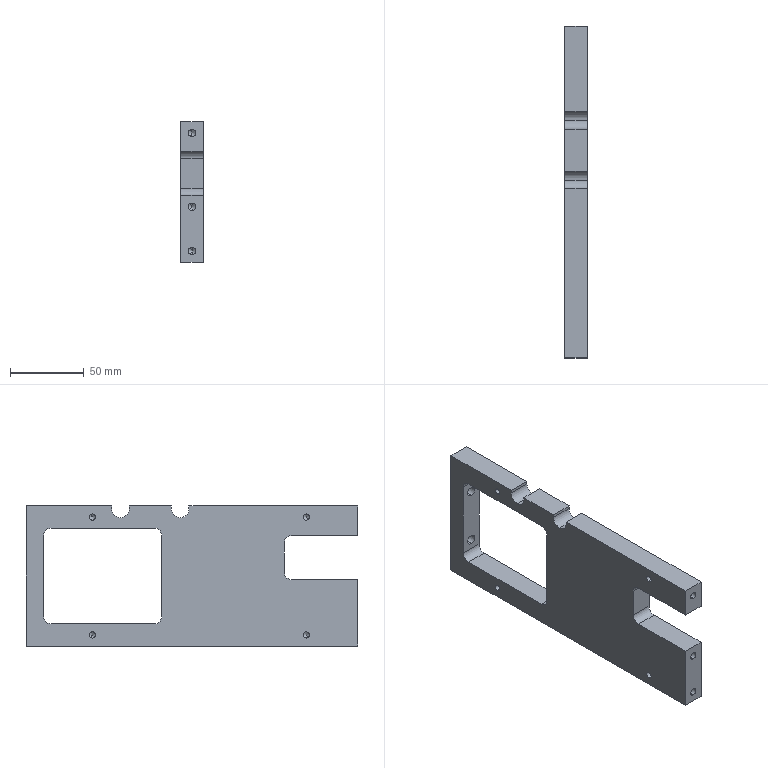Part | SolidWorks | features HoleWzd 5, Cut 2, Extrusion 1, ICE 1, MirrorPattern 1 | 1 solid | 70 faces | box 15 x 225.1 x 95 mm | volume 215693 mm3 | cylinder 32 | plane 20 | cone 18 | commonest cylinder face diameters 5 x10 4.2 x8 10 x6 6.6 x4 12 x4